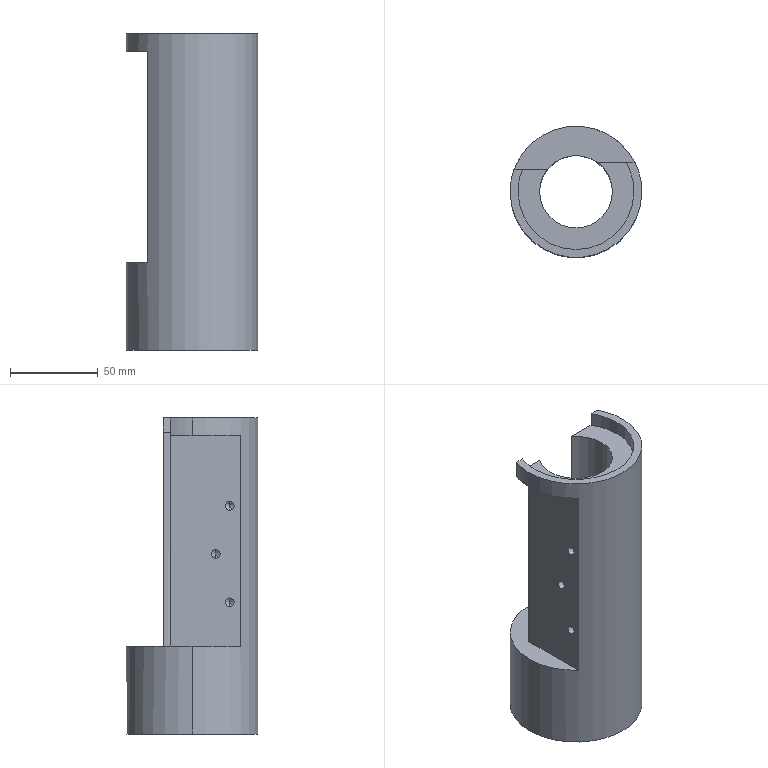Part | STEP file | Round guide sleeve SGN-2-10 | 1 solid | 31 faces | box 75 x 75 x 180 mm | volume 346678 mm3 | cylinder 16 | plane 9 | cone 6 | commonest cylinder face diameters 5 x6 66 x5 75 x3 41.5 x2